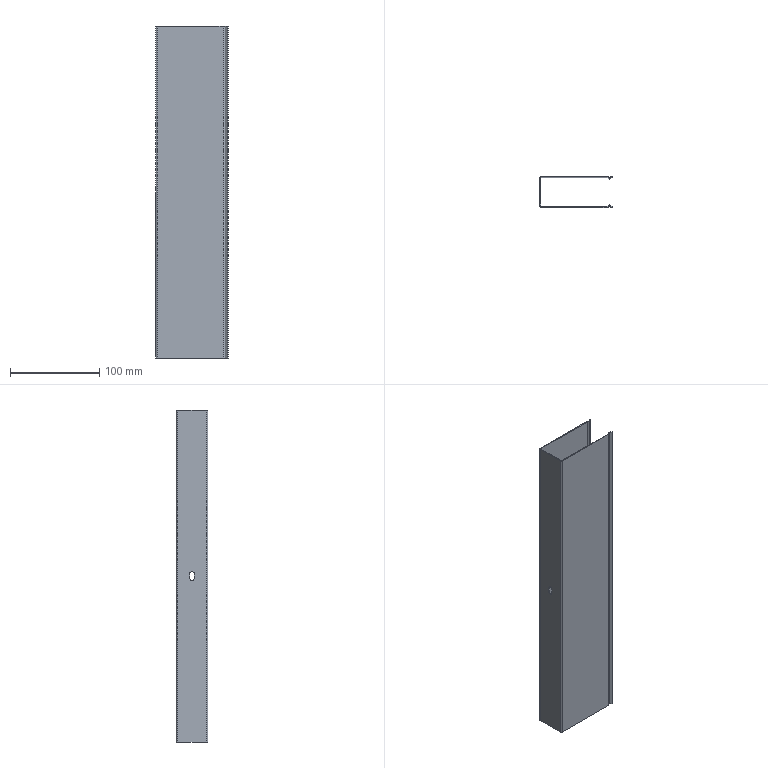Part | STEP file | 1 solid | 27 faces | box 80.625 x 35 x 371 mm | volume 72614 mm3 | plane 20 | cylinder 7 | commonest cylinder face diameters 5 x3 1 x2 3 x2